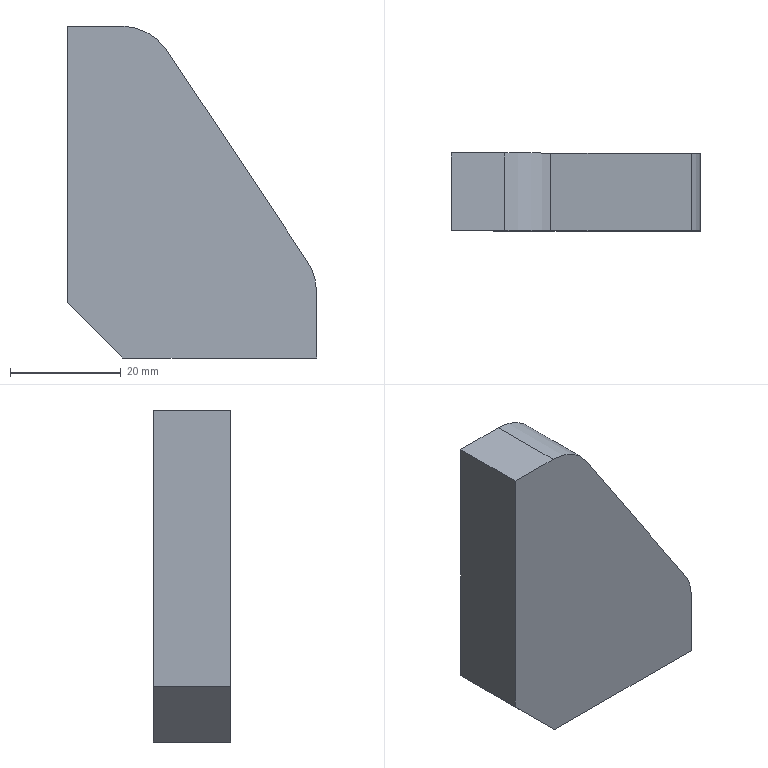Part | SolidWorks | features BaseBody 1 | 1 solid | 10 faces | box 45 x 14 x 60 mm | volume 27576 mm3 | plane 8 | cylinder 2 | commonest cylinder face diameters 20 x2
STEP:
#1=CARTESIAN_POINT('',(22.5,-7.,-18.028));
#2=VERTEX_POINT('',#1);
#3=CARTESIAN_POINT('',(22.5,-7.,-30.));
#4=VERTEX_POINT('',#3);
#5=CARTESIAN_POINT('',(22.5,-7.,-18.028));
#6=DIRECTION('',(0.,0.,-1.));
#7=VECTOR('',#6,1000.);
#8=LINE('',#5,#7);
#9=EDGE_CURVE('',#2,#4,#8,.T.);
#10=ORIENTED_EDGE('',*,*,#9,.T.);
#11=CARTESIAN_POINT('',(22.5,7.,-30.));
#12=VERTEX_POINT('',#11);
#13=CARTESIAN_POINT('',(22.5,7.,-30.));
#14=DIRECTION('',(0.,-1.,0.));
#15=VECTOR('',#14,1000.);
#16=LINE('',#13,#15);
#17=EDGE_CURVE('',#12,#4,#16,.T.);
#18=ORIENTED_EDGE('',*,*,#17,.F.);
#19=CARTESIAN_POINT('',(22.5,7.,-18.028));
#20=VERTEX_POINT('',#19);
#21=CARTESIAN_POINT('',(22.5,7.,-18.028));
#22=DIRECTION('',(0.,0.,-1.));
#23=VECTOR('',#22,1000.);
#24=LINE('',#21,#23);
#25=EDGE_CURVE('',#20,#12,#24,.T.);
#26=ORIENTED_EDGE('',*,*,#25,.F.);
#27=CARTESIAN_POINT('',(22.5,7.,-18.028));
#28=DIRECTION('',(0.,-1.,0.));
#29=VECTOR('',#28,1000.);
#30=LINE('',#27,#29);
#31=EDGE_CURVE('',#20,#2,#30,.T.);
#32=ORIENTED_EDGE('',*,*,#31,.T.);
#33=EDGE_LOOP('',(#10,#18,#26,#32));
#34=FACE_OUTER_BOUND('',#33,.T.);
#35=CARTESIAN_POINT('',(22.5,7.,-18.028));
#36=DIRECTION('',(-1.,0.,0.));
#37=DIRECTION('',(0.,0.,1.));
#38=AXIS2_PLACEMENT_3D('',#35,#36,#37);
#39=PLANE('',#38);
#40=ADVANCED_FACE('',(#34),#39,.F.);
#41=CARTESIAN_POINT('',(-12.5,-7.,-30.));
#42=VERTEX_POINT('',#41);
#43=CARTESIAN_POINT('',(22.5,-7.,-30.));
#44=DIRECTION('',(-1.,0.,0.));
#45=VECTOR('',#44,1000.);
#46=LINE('',#43,#45);
#47=EDGE_CURVE('',#4,#42,#46,.T.);
#48=ORIENTED_EDGE('',*,*,#47,.T.);
#49=CARTESIAN_POINT('',(-12.5,7.,-30.));
#50=VERTEX_POINT('',#49);
#51=CARTESIAN_POINT('',(-12.5,7.,-30.));
#52=DIRECTION('',(0.,-1.,0.));
#53=VECTOR('',#52,1000.);
#54=LINE('',#51,#53);
#55=EDGE_CURVE('',#50,#42,#54,.T.);
#56=ORIENTED_EDGE('',*,*,#55,.F.);
#57=CARTESIAN_POINT('',(22.5,7.,-30.));
#58=DIRECTION('',(-1.,0.,0.));
#59=VECTOR('',#58,1000.);
#60=LINE('',#57,#59);
#61=EDGE_CURVE('',#12,#50,#60,.T.);
#62=ORIENTED_EDGE('',*,*,#61,.F.);
#63=ORIENTED_EDGE('',*,*,#17,.T.);
#64=EDGE_LOOP('',(#48,#56,#62,#63));
#65=FACE_OUTER_BOUND('',#64,.T.);
#66=CARTESIAN_POINT('',(22.5,7.,-30.));
#67=DIRECTION('',(0.,0.,1.));
#68=DIRECTION('',(1.,0.,0.));
#69=AXIS2_PLACEMENT_3D('',#66,#67,#68);
#70=PLANE('',#69);
#71=ADVANCED_FACE('',(#65),#70,.F.);
#72=CARTESIAN_POINT('',(-22.5,-7.,-20.));
#73=VERTEX_POINT('',#72);
#74=CARTESIAN_POINT('',(-12.5,-7.,-30.));
#75=DIRECTION('',(-0.7071,0.,0.7071));
#76=VECTOR('',#75,1000.);
#77=LINE('',#74,#76);
#78=EDGE_CURVE('',#42,#73,#77,.T.);
#79=ORIENTED_EDGE('',*,*,#78,.T.);
#80=CARTESIAN_POINT('',(-22.5,7.,-20.));
#81=VERTEX_POINT('',#80);
#82=CARTESIAN_POINT('',(-22.5,7.,-20.));
#83=DIRECTION('',(0.,-1.,0.));
#84=VECTOR('',#83,1000.);
#85=LINE('',#82,#84);
#86=EDGE_CURVE('',#81,#73,#85,.T.);
#87=ORIENTED_EDGE('',*,*,#86,.F.);
#88=CARTESIAN_POINT('',(-12.5,7.,-30.));
#89=DIRECTION('',(-0.7071,0.,0.7071));
#90=VECTOR('',#89,1000.);
#91=LINE('',#88,#90);
#92=EDGE_CURVE('',#50,#81,#91,.T.);
#93=ORIENTED_EDGE('',*,*,#92,.F.);
#94=ORIENTED_EDGE('',*,*,#55,.T.);
#95=EDGE_LOOP('',(#79,#87,#93,#94));
#96=FACE_OUTER_BOUND('',#95,.T.);
#97=CARTESIAN_POINT('',(-12.5,7.,-30.));
#98=DIRECTION('',(0.7071,0.,0.7071));
#99=DIRECTION('',(0.7071,0.,-0.7071));
#100=AXIS2_PLACEMENT_3D('',#97,#98,#99);
#101=PLANE('',#100);
#102=ADVANCED_FACE('',(#96),#101,.F.);
#103=CARTESIAN_POINT('',(-22.5,-7.,30.));
#104=VERTEX_POINT('',#103);
#105=CARTESIAN_POINT('',(-22.5,-7.,-20.));
#106=DIRECTION('',(0.,0.,1.));
#107=VECTOR('',#106,1000.);
#108=LINE('',#105,#107);
#109=EDGE_CURVE('',#73,#104,#108,.T.);
#110=ORIENTED_EDGE('',*,*,#109,.T.);
#111=CARTESIAN_POINT('',(-22.5,7.,30.));
#112=VERTEX_POINT('',#111);
#113=CARTESIAN_POINT('',(-22.5,7.,30.));
#114=DIRECTION('',(0.,-1.,0.));
#115=VECTOR('',#114,1000.);
#116=LINE('',#113,#115);
#117=EDGE_CURVE('',#112,#104,#116,.T.);
#118=ORIENTED_EDGE('',*,*,#117,.F.);
#119=CARTESIAN_POINT('',(-22.5,7.,-20.));
#120=DIRECTION('',(0.,0.,1.));
#121=VECTOR('',#120,1000.);
#122=LINE('',#119,#121);
#123=EDGE_CURVE('',#81,#112,#122,.T.);
#124=ORIENTED_EDGE('',*,*,#123,.F.);
#125=ORIENTED_EDGE('',*,*,#86,.T.);
#126=EDGE_LOOP('',(#110,#118,#124,#125));
#127=FACE_OUTER_BOUND('',#126,.T.);
#128=CARTESIAN_POINT('',(-22.5,7.,-20.));
#129=DIRECTION('',(1.,0.,0.));
#130=DIRECTION('',(0.,0.,-1.));
#131=AXIS2_PLACEMENT_3D('',#128,#129,#130);
#132=PLANE('',#131);
#133=ADVANCED_FACE('',(#127),#132,.F.);
#134=CARTESIAN_POINT('',(-12.852,-7.,30.));
#135=VERTEX_POINT('',#134);
#136=CARTESIAN_POINT('',(-22.5,-7.,30.));
#137=DIRECTION('',(1.,0.,0.));
#138=VECTOR('',#137,1000.);
#139=LINE('',#136,#138);
#140=EDGE_CURVE('',#104,#135,#139,.T.);
#141=ORIENTED_EDGE('',*,*,#140,.T.);
#142=CARTESIAN_POINT('',(-12.852,7.,30.));
#143=VERTEX_POINT('',#142);
#144=CARTESIAN_POINT('',(-12.852,7.,30.));
#145=DIRECTION('',(0.,-1.,0.));
#146=VECTOR('',#145,1000.);
#147=LINE('',#144,#146);
#148=EDGE_CURVE('',#143,#135,#147,.T.);
#149=ORIENTED_EDGE('',*,*,#148,.F.);
#150=CARTESIAN_POINT('',(-22.5,7.,30.));
#151=DIRECTION('',(1.,0.,0.));
#152=VECTOR('',#151,1000.);
#153=LINE('',#150,#152);
#154=EDGE_CURVE('',#112,#143,#153,.T.);
#155=ORIENTED_EDGE('',*,*,#154,.F.);
#156=ORIENTED_EDGE('',*,*,#117,.T.);
#157=EDGE_LOOP('',(#141,#149,#155,#156));
#158=FACE_OUTER_BOUND('',#157,.T.);
#159=CARTESIAN_POINT('',(-22.5,7.,30.));
#160=DIRECTION('',(0.,0.,-1.));
#161=DIRECTION('',(-1.,0.,0.));
#162=AXIS2_PLACEMENT_3D('',#159,#160,#161);
#163=PLANE('',#162);
#164=ADVANCED_FACE('',(#158),#163,.F.);
#165=CARTESIAN_POINT('',(-4.531,-7.,25.547));
#166=VERTEX_POINT('',#165);
#167=CARTESIAN_POINT('',(-12.852,-7.,20.));
#168=DIRECTION('',(0.,1.,0.));
#169=DIRECTION('',(0.,0.,1.));
#170=AXIS2_PLACEMENT_3D('',#167,#168,#169);
#171=CIRCLE('',#170,10.);
#172=EDGE_CURVE('',#135,#166,#171,.T.);
#173=ORIENTED_EDGE('',*,*,#172,.T.);
#174=CARTESIAN_POINT('',(-4.531,7.,25.547));
#175=VERTEX_POINT('',#174);
#176=CARTESIAN_POINT('',(-4.531,7.,25.547));
#177=DIRECTION('',(0.,-1.,0.));
#178=VECTOR('',#177,1000.);
#179=LINE('',#176,#178);
#180=EDGE_CURVE('',#175,#166,#179,.T.);
#181=ORIENTED_EDGE('',*,*,#180,.F.);
#182=CARTESIAN_POINT('',(-12.852,7.,20.));
#183=DIRECTION('',(0.,1.,0.));
#184=DIRECTION('',(0.,0.,1.));
#185=AXIS2_PLACEMENT_3D('',#182,#183,#184);
#186=CIRCLE('',#185,10.);
#187=EDGE_CURVE('',#143,#175,#186,.T.);
#188=ORIENTED_EDGE('',*,*,#187,.F.);
#189=ORIENTED_EDGE('',*,*,#148,.T.);
#190=EDGE_LOOP('',(#173,#181,#188,#189));
#191=FACE_OUTER_BOUND('',#190,.T.);
#192=CARTESIAN_POINT('',(-12.852,7.,20.));
#193=DIRECTION('',(0.,-1.,0.));
#194=DIRECTION('',(0.,0.,-1.));
#195=AXIS2_PLACEMENT_3D('',#192,#193,#194);
#196=CYLINDRICAL_SURFACE('',#195,10.);
#197=ADVANCED_FACE('',(#191),#196,.T.);
#198=CARTESIAN_POINT('',(20.821,-7.,-12.481));
#199=VERTEX_POINT('',#198);
#200=CARTESIAN_POINT('',(-4.531,-7.,25.547));
#201=DIRECTION('',(0.5547,0.,-0.8321));
#202=VECTOR('',#201,1000.);
#203=LINE('',#200,#202);
#204=EDGE_CURVE('',#166,#199,#203,.T.);
#205=ORIENTED_EDGE('',*,*,#204,.T.);
#206=CARTESIAN_POINT('',(20.821,7.,-12.481));
#207=VERTEX_POINT('',#206);
#208=CARTESIAN_POINT('',(20.821,7.,-12.481));
#209=DIRECTION('',(0.,-1.,0.));
#210=VECTOR('',#209,1000.);
#211=LINE('',#208,#210);
#212=EDGE_CURVE('',#207,#199,#211,.T.);
#213=ORIENTED_EDGE('',*,*,#212,.F.);
#214=CARTESIAN_POINT('',(-4.531,7.,25.547));
#215=DIRECTION('',(0.5547,0.,-0.8321));
#216=VECTOR('',#215,1000.);
#217=LINE('',#214,#216);
#218=EDGE_CURVE('',#175,#207,#217,.T.);
#219=ORIENTED_EDGE('',*,*,#218,.F.);
#220=ORIENTED_EDGE('',*,*,#180,.T.);
#221=EDGE_LOOP('',(#205,#213,#219,#220));
#222=FACE_OUTER_BOUND('',#221,.T.);
#223=CARTESIAN_POINT('',(-4.531,7.,25.547));
#224=DIRECTION('',(-0.8321,0.,-0.5547));
#225=DIRECTION('',(-0.5547,0.,0.8321));
#226=AXIS2_PLACEMENT_3D('',#223,#224,#225);
#227=PLANE('',#226);
#228=ADVANCED_FACE('',(#222),#227,.F.);
#229=CARTESIAN_POINT('',(12.5,-7.,-18.028));
#230=DIRECTION('',(0.,1.,0.));
#231=DIRECTION('',(0.,0.,1.));
#232=AXIS2_PLACEMENT_3D('',#229,#230,#231);
#233=CIRCLE('',#232,10.);
#234=EDGE_CURVE('',#199,#2,#233,.T.);
#235=ORIENTED_EDGE('',*,*,#234,.T.);
#236=ORIENTED_EDGE('',*,*,#31,.F.);
#237=CARTESIAN_POINT('',(12.5,7.,-18.028));
#238=DIRECTION('',(0.,1.,0.));
#239=DIRECTION('',(0.,0.,1.));
#240=AXIS2_PLACEMENT_3D('',#237,#238,#239);
#241=CIRCLE('',#240,10.);
#242=EDGE_CURVE('',#207,#20,#241,.T.);
#243=ORIENTED_EDGE('',*,*,#242,.F.);
#244=ORIENTED_EDGE('',*,*,#212,.T.);
#245=EDGE_LOOP('',(#235,#236,#243,#244));
#246=FACE_OUTER_BOUND('',#245,.T.);
#247=CARTESIAN_POINT('',(12.5,7.,-18.028));
#248=DIRECTION('',(0.,-1.,0.));
#249=DIRECTION('',(0.,0.,-1.));
#250=AXIS2_PLACEMENT_3D('',#247,#248,#249);
#251=CYLINDRICAL_SURFACE('',#250,10.);
#252=ADVANCED_FACE('',(#246),#251,.T.);
#253=ORIENTED_EDGE('',*,*,#25,.T.);
#254=ORIENTED_EDGE('',*,*,#61,.T.);
#255=ORIENTED_EDGE('',*,*,#92,.T.);
#256=ORIENTED_EDGE('',*,*,#123,.T.);
#257=ORIENTED_EDGE('',*,*,#154,.T.);
#258=ORIENTED_EDGE('',*,*,#187,.T.);
#259=ORIENTED_EDGE('',*,*,#218,.T.);
#260=ORIENTED_EDGE('',*,*,#242,.T.);
#261=EDGE_LOOP('',(#253,#254,#255,#256,#257,#258,#259,#260));
#262=FACE_OUTER_BOUND('',#261,.T.);
#263=CARTESIAN_POINT('',(-12.852,7.,20.));
#264=DIRECTION('',(0.,1.,0.));
#265=DIRECTION('',(0.,0.,1.));
#266=AXIS2_PLACEMENT_3D('',#263,#264,#265);
#267=PLANE('',#266);
#268=ADVANCED_FACE('',(#262),#267,.T.);
#269=ORIENTED_EDGE('',*,*,#9,.F.);
#270=ORIENTED_EDGE('',*,*,#234,.F.);
#271=ORIENTED_EDGE('',*,*,#204,.F.);
#272=ORIENTED_EDGE('',*,*,#172,.F.);
#273=ORIENTED_EDGE('',*,*,#140,.F.);
#274=ORIENTED_EDGE('',*,*,#109,.F.);
#275=ORIENTED_EDGE('',*,*,#78,.F.);
#276=ORIENTED_EDGE('',*,*,#47,.F.);
#277=EDGE_LOOP('',(#269,#270,#271,#272,#273,#274,#275,#276));
#278=FACE_OUTER_BOUND('',#277,.T.);
#279=CARTESIAN_POINT('',(-12.852,-7.,20.));
#280=DIRECTION('',(0.,1.,0.));
#281=DIRECTION('',(0.,0.,1.));
#282=AXIS2_PLACEMENT_3D('',#279,#280,#281);
#283=PLANE('',#282);
#284=ADVANCED_FACE('',(#278),#283,.F.);
#285=CLOSED_SHELL('',(#40,#71,#102,#133,#164,#197,#228,#252,#268,#284));
#286=MANIFOLD_SOLID_BREP('',#285);
#287=CARTESIAN_POINT('',(0.,0.,0.));
#288=DIRECTION('',(0.,0.,1.));
#289=DIRECTION('',(1.,0.,0.));
#290=AXIS2_PLACEMENT_3D('',#287,#288,#289);
#291=(LENGTH_UNIT()NAMED_UNIT(*)SI_UNIT(.MILLI.,.METRE.));
#292=UNCERTAINTY_MEASURE_WITH_UNIT(LENGTH_MEASURE(0.00001),#291,'','');
#293=(NAMED_UNIT(*)PLANE_ANGLE_UNIT()SI_UNIT($,.RADIAN.));
#294=(NAMED_UNIT(*)SI_UNIT($,.STERADIAN.)SOLID_ANGLE_UNIT());
#295=(GEOMETRIC_REPRESENTATION_CONTEXT(3)GLOBAL_UNCERTAINTY_ASSIGNED_CONTEXT((#292))GLOBAL_UNIT_ASSIGNED_CONTEXT((#291,#293,#294))REPRESENTATION_CONTEXT('',''));
#296=ADVANCED_BREP_SHAPE_REPRESENTATION('',(#286,#290),#295);